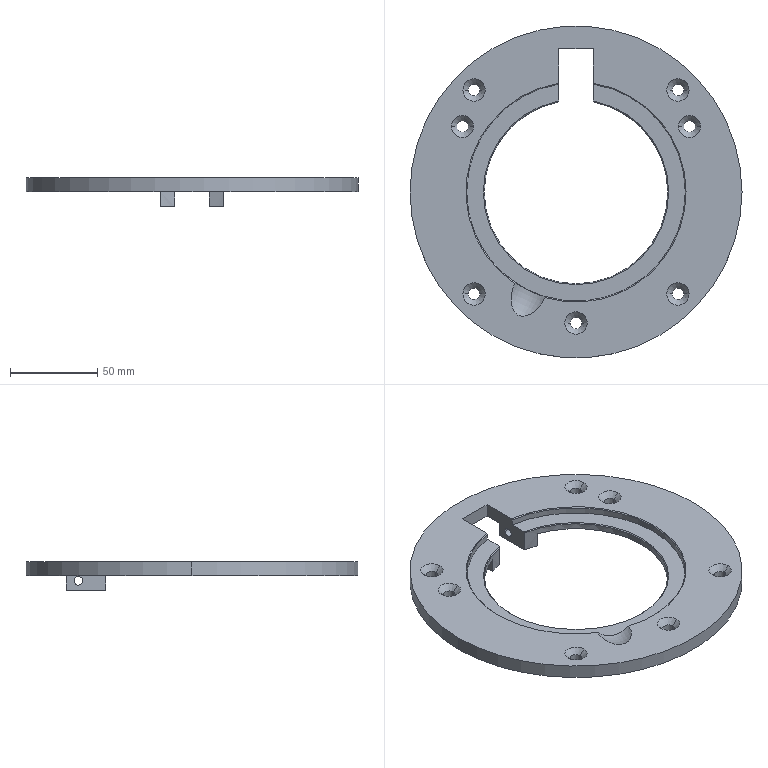Part | SolidWorks | features ICE 4, 3DProfileFeature 2, CirPattern 2, HoleWzd 2, Chamfer 1, Extrusion 1, RevCut 1 | 1 solid | 59 faces | box 190 x 190 x 16.5 mm | volume 138336 mm3 | cylinder 26 | cone 20 | plane 12 | torus 1 | commonest cylinder face diameters 6.6 x14 5 x4 105 x3 125 x3 190 x2